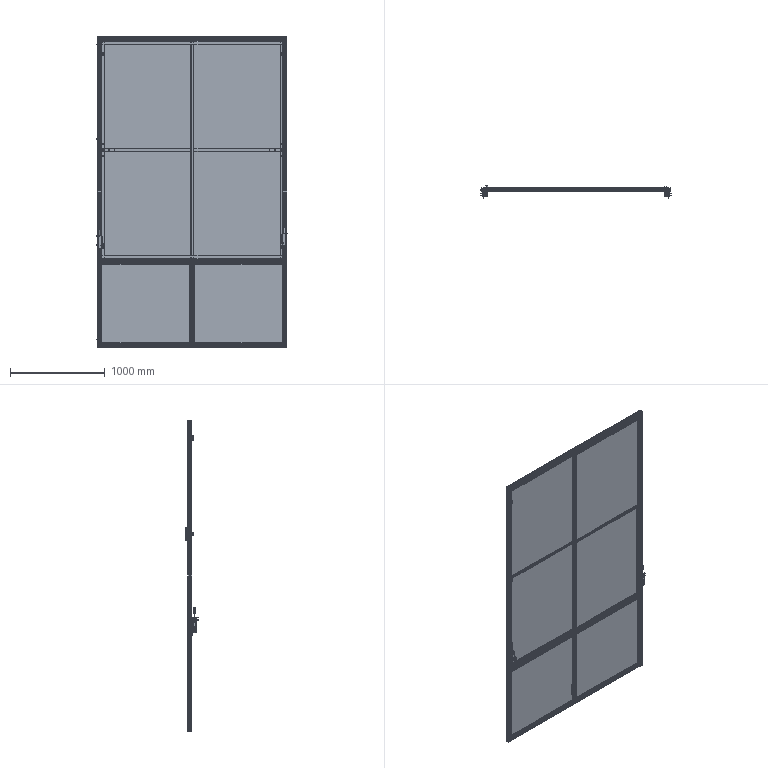Part | SolidWorks | 244 solids | 16446 faces | volume 41950678 mm3 | plane 8766 | cylinder 4332 | cone 2100 | spline 710 | torus 446 | sphere 92 | commonest cylinder face diameters 1 x446 2.5 x356 5 x318 2 x300 0.4 x184 4.5 x178